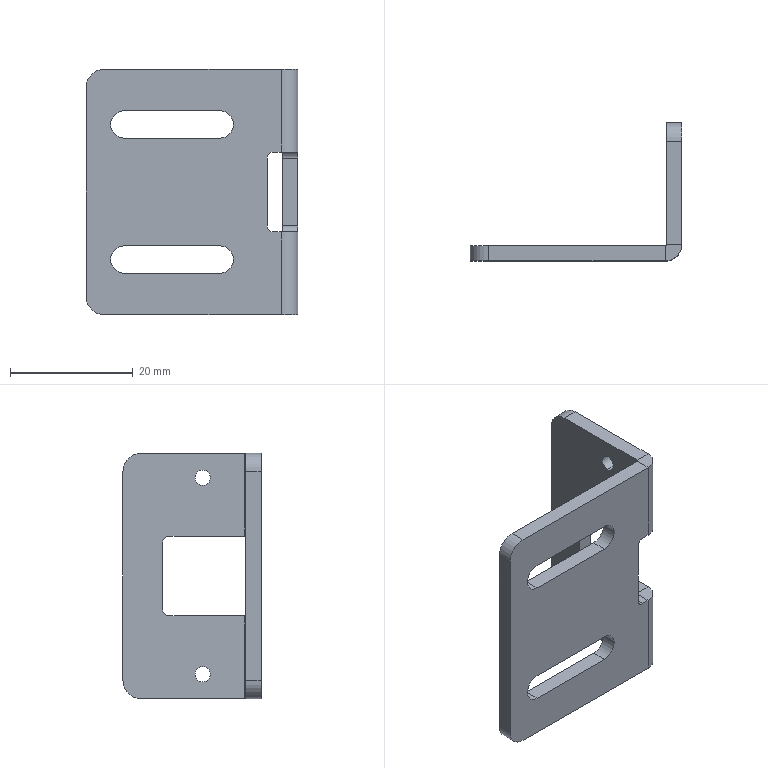Part | STEP file | 1 solid | 44 faces | box 34.5 x 22.5 x 40 mm | volume 4337 mm3 | plane 24 | cylinder 20 | commonest cylinder face diameters 2 x4 2.5 x4 4.5 x4 6 x4 0.4 x2 5.4 x2